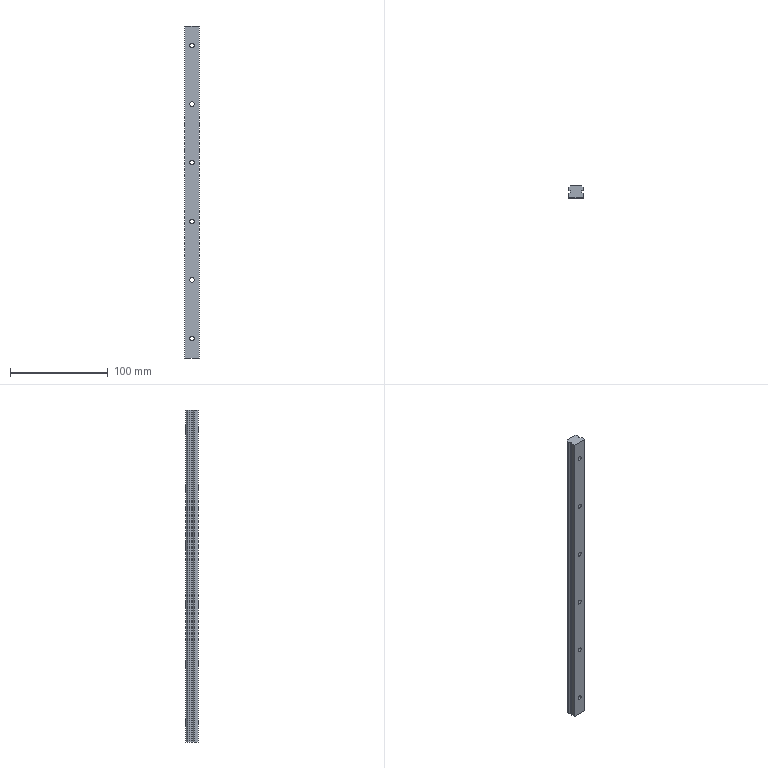Part | NX | features BREP 1 | 1 solid | 46 faces | box 15 x 12.5 x 340 mm | volume 57238 mm3 | cylinder 24 | plane 22 | commonest cylinder face diameters 4.5 x12 7.5 x12
STEP:
#1=CARTESIAN_POINT('',(-78.,48.25,170.));
#2=VERTEX_POINT('',#1);
#3=CARTESIAN_POINT('',(-80.,46.25,170.));
#4=VERTEX_POINT('',#3);
#5=CARTESIAN_POINT('',(-80.,46.25,170.));
#6=DIRECTION('',(-0.7071,-0.7071,0.));
#7=VECTOR('',#6,1000.);
#8=LINE('',#5,#7);
#9=EDGE_CURVE('',#2,#4,#8,.T.);
#10=ORIENTED_EDGE('',*,*,#9,.F.);
#11=CARTESIAN_POINT('',(-78.,48.25,-170.));
#12=VERTEX_POINT('',#11);
#13=CARTESIAN_POINT('',(-78.,48.25,170.));
#14=DIRECTION('',(0.,0.,1.));
#15=VECTOR('',#14,1000.);
#16=LINE('',#13,#15);
#17=EDGE_CURVE('',#12,#2,#16,.T.);
#18=ORIENTED_EDGE('',*,*,#17,.F.);
#19=CARTESIAN_POINT('',(-80.,46.25,-170.));
#20=VERTEX_POINT('',#19);
#21=CARTESIAN_POINT('',(-78.375,47.875,-170.));
#22=DIRECTION('',(0.7071,0.7071,0.));
#23=VECTOR('',#22,1000.);
#24=LINE('',#21,#23);
#25=EDGE_CURVE('',#20,#12,#24,.T.);
#26=ORIENTED_EDGE('',*,*,#25,.F.);
#27=CARTESIAN_POINT('',(-80.,46.25,170.));
#28=DIRECTION('',(0.,0.,-1.));
#29=VECTOR('',#28,1000.);
#30=LINE('',#27,#29);
#31=EDGE_CURVE('',#4,#20,#30,.T.);
#32=ORIENTED_EDGE('',*,*,#31,.F.);
#33=EDGE_LOOP('',(#10,#18,#26,#32));
#34=FACE_BOUND('',#33,.T.);
#35=CARTESIAN_POINT('',(-80.,46.25,170.));
#36=DIRECTION('',(0.7071,-0.7071,0.));
#37=DIRECTION('',(0.,0.,-1.));
#38=AXIS2_PLACEMENT_3D('',#35,#36,#37);
#39=PLANE('',#38);
#40=ADVANCED_FACE('',(#34),#39,.F.);
#41=CARTESIAN_POINT('',(-65.,46.25,170.));
#42=VERTEX_POINT('',#41);
#43=CARTESIAN_POINT('',(-67.,48.25,170.));
#44=VERTEX_POINT('',#43);
#45=CARTESIAN_POINT('',(-67.,48.25,170.));
#46=DIRECTION('',(-0.7071,0.7071,0.));
#47=VECTOR('',#46,1000.);
#48=LINE('',#45,#47);
#49=EDGE_CURVE('',#42,#44,#48,.T.);
#50=ORIENTED_EDGE('',*,*,#49,.F.);
#51=CARTESIAN_POINT('',(-65.,46.25,-170.));
#52=VERTEX_POINT('',#51);
#53=CARTESIAN_POINT('',(-65.,46.25,170.));
#54=DIRECTION('',(0.,0.,1.));
#55=VECTOR('',#54,1000.);
#56=LINE('',#53,#55);
#57=EDGE_CURVE('',#52,#42,#56,.T.);
#58=ORIENTED_EDGE('',*,*,#57,.F.);
#59=CARTESIAN_POINT('',(-67.,48.25,-170.));
#60=VERTEX_POINT('',#59);
#61=CARTESIAN_POINT('',(-66.625,47.875,-170.));
#62=DIRECTION('',(0.7071,-0.7071,0.));
#63=VECTOR('',#62,1000.);
#64=LINE('',#61,#63);
#65=EDGE_CURVE('',#60,#52,#64,.T.);
#66=ORIENTED_EDGE('',*,*,#65,.F.);
#67=CARTESIAN_POINT('',(-67.,48.25,170.));
#68=DIRECTION('',(0.,0.,-1.));
#69=VECTOR('',#68,1000.);
#70=LINE('',#67,#69);
#71=EDGE_CURVE('',#44,#60,#70,.T.);
#72=ORIENTED_EDGE('',*,*,#71,.F.);
#73=EDGE_LOOP('',(#50,#58,#66,#72));
#74=FACE_BOUND('',#73,.T.);
#75=CARTESIAN_POINT('',(-67.,48.25,170.));
#76=DIRECTION('',(-0.7071,-0.7071,0.));
#77=DIRECTION('',(0.,0.,-1.));
#78=AXIS2_PLACEMENT_3D('',#75,#76,#77);
#79=PLANE('',#78);
#80=ADVANCED_FACE('',(#74),#79,.F.);
#81=CARTESIAN_POINT('',(-66.5,42.75,170.));
#82=VERTEX_POINT('',#81);
#83=CARTESIAN_POINT('',(-66.5,41.25,170.));
#84=VERTEX_POINT('',#83);
#85=CARTESIAN_POINT('',(-66.5,41.25,170.));
#86=DIRECTION('',(0.,-1.,0.));
#87=VECTOR('',#86,1000.);
#88=LINE('',#85,#87);
#89=EDGE_CURVE('',#82,#84,#88,.T.);
#90=ORIENTED_EDGE('',*,*,#89,.T.);
#91=CARTESIAN_POINT('',(-66.5,41.25,-170.));
#92=VERTEX_POINT('',#91);
#93=CARTESIAN_POINT('',(-66.5,41.25,-170.));
#94=DIRECTION('',(0.,0.,1.));
#95=VECTOR('',#94,1000.);
#96=LINE('',#93,#95);
#97=EDGE_CURVE('',#92,#84,#96,.T.);
#98=ORIENTED_EDGE('',*,*,#97,.F.);
#99=CARTESIAN_POINT('',(-66.5,42.75,-170.));
#100=VERTEX_POINT('',#99);
#101=CARTESIAN_POINT('',(-66.5,41.25,-170.));
#102=DIRECTION('',(0.,-1.,0.));
#103=VECTOR('',#102,1000.);
#104=LINE('',#101,#103);
#105=EDGE_CURVE('',#100,#92,#104,.T.);
#106=ORIENTED_EDGE('',*,*,#105,.F.);
#107=CARTESIAN_POINT('',(-66.5,42.75,-170.));
#108=DIRECTION('',(0.,0.,1.));
#109=VECTOR('',#108,1000.);
#110=LINE('',#107,#109);
#111=EDGE_CURVE('',#100,#82,#110,.T.);
#112=ORIENTED_EDGE('',*,*,#111,.T.);
#113=EDGE_LOOP('',(#90,#98,#106,#112));
#114=FACE_BOUND('',#113,.T.);
#115=CARTESIAN_POINT('',(-66.5,41.25,-170.));
#116=DIRECTION('',(-1.,0.,0.));
#117=DIRECTION('',(0.,-1.,0.));
#118=AXIS2_PLACEMENT_3D('',#115,#116,#117);
#119=PLANE('',#118);
#120=ADVANCED_FACE('',(#114),#119,.F.);
#121=CARTESIAN_POINT('',(-65.,39.75,170.));
#122=VERTEX_POINT('',#121);
#123=CARTESIAN_POINT('',(-65.,39.75,170.));
#124=DIRECTION('',(0.7071,-0.7071,0.));
#125=VECTOR('',#124,1000.);
#126=LINE('',#123,#125);
#127=EDGE_CURVE('',#84,#122,#126,.T.);
#128=ORIENTED_EDGE('',*,*,#127,.T.);
#129=CARTESIAN_POINT('',(-65.,39.75,-170.));
#130=VERTEX_POINT('',#129);
#131=CARTESIAN_POINT('',(-65.,39.75,-170.));
#132=DIRECTION('',(0.,0.,1.));
#133=VECTOR('',#132,1000.);
#134=LINE('',#131,#133);
#135=EDGE_CURVE('',#130,#122,#134,.T.);
#136=ORIENTED_EDGE('',*,*,#135,.F.);
#137=CARTESIAN_POINT('',(-65.,39.75,-170.));
#138=DIRECTION('',(0.7071,-0.7071,0.));
#139=VECTOR('',#138,1000.);
#140=LINE('',#137,#139);
#141=EDGE_CURVE('',#92,#130,#140,.T.);
#142=ORIENTED_EDGE('',*,*,#141,.F.);
#143=ORIENTED_EDGE('',*,*,#97,.T.);
#144=EDGE_LOOP('',(#128,#136,#142,#143));
#145=FACE_BOUND('',#144,.T.);
#146=CARTESIAN_POINT('',(-65.,39.75,-170.));
#147=DIRECTION('',(-0.7071,-0.7071,0.));
#148=DIRECTION('',(0.7071,-0.7071,0.));
#149=AXIS2_PLACEMENT_3D('',#146,#147,#148);
#150=PLANE('',#149);
#151=ADVANCED_FACE('',(#145),#150,.F.);
#152=CARTESIAN_POINT('',(-65.,44.25,170.));
#153=VERTEX_POINT('',#152);
#154=CARTESIAN_POINT('',(-66.5,42.75,170.));
#155=DIRECTION('',(-0.7071,-0.7071,0.));
#156=VECTOR('',#155,1000.);
#157=LINE('',#154,#156);
#158=EDGE_CURVE('',#153,#82,#157,.T.);
#159=ORIENTED_EDGE('',*,*,#158,.T.);
#160=ORIENTED_EDGE('',*,*,#111,.F.);
#161=CARTESIAN_POINT('',(-65.,44.25,-170.));
#162=VERTEX_POINT('',#161);
#163=CARTESIAN_POINT('',(-66.5,42.75,-170.));
#164=DIRECTION('',(-0.7071,-0.7071,0.));
#165=VECTOR('',#164,1000.);
#166=LINE('',#163,#165);
#167=EDGE_CURVE('',#162,#100,#166,.T.);
#168=ORIENTED_EDGE('',*,*,#167,.F.);
#169=CARTESIAN_POINT('',(-65.,44.25,-170.));
#170=DIRECTION('',(0.,0.,1.));
#171=VECTOR('',#170,1000.);
#172=LINE('',#169,#171);
#173=EDGE_CURVE('',#162,#153,#172,.T.);
#174=ORIENTED_EDGE('',*,*,#173,.T.);
#175=EDGE_LOOP('',(#159,#160,#168,#174));
#176=FACE_BOUND('',#175,.T.);
#177=CARTESIAN_POINT('',(-66.5,42.75,-170.));
#178=DIRECTION('',(-0.7071,0.7071,0.));
#179=DIRECTION('',(-0.7071,-0.7071,0.));
#180=AXIS2_PLACEMENT_3D('',#177,#178,#179);
#181=PLANE('',#180);
#182=ADVANCED_FACE('',(#176),#181,.F.);
#183=CARTESIAN_POINT('',(-80.,39.75,170.));
#184=VERTEX_POINT('',#183);
#185=CARTESIAN_POINT('',(-78.5,41.25,170.));
#186=VERTEX_POINT('',#185);
#187=CARTESIAN_POINT('',(-80.,39.75,170.));
#188=DIRECTION('',(0.7071,0.7071,0.));
#189=VECTOR('',#188,1000.);
#190=LINE('',#187,#189);
#191=EDGE_CURVE('',#184,#186,#190,.T.);
#192=ORIENTED_EDGE('',*,*,#191,.T.);
#193=CARTESIAN_POINT('',(-78.5,41.25,-170.));
#194=VERTEX_POINT('',#193);
#195=CARTESIAN_POINT('',(-78.5,41.25,-170.));
#196=DIRECTION('',(0.,0.,1.));
#197=VECTOR('',#196,1000.);
#198=LINE('',#195,#197);
#199=EDGE_CURVE('',#194,#186,#198,.T.);
#200=ORIENTED_EDGE('',*,*,#199,.F.);
#201=CARTESIAN_POINT('',(-80.,39.75,-170.));
#202=VERTEX_POINT('',#201);
#203=CARTESIAN_POINT('',(-80.,39.75,-170.));
#204=DIRECTION('',(0.7071,0.7071,0.));
#205=VECTOR('',#204,1000.);
#206=LINE('',#203,#205);
#207=EDGE_CURVE('',#202,#194,#206,.T.);
#208=ORIENTED_EDGE('',*,*,#207,.F.);
#209=CARTESIAN_POINT('',(-80.,39.75,-170.));
#210=DIRECTION('',(0.,0.,1.));
#211=VECTOR('',#210,1000.);
#212=LINE('',#209,#211);
#213=EDGE_CURVE('',#202,#184,#212,.T.);
#214=ORIENTED_EDGE('',*,*,#213,.T.);
#215=EDGE_LOOP('',(#192,#200,#208,#214));
#216=FACE_BOUND('',#215,.T.);
#217=CARTESIAN_POINT('',(-80.,39.75,-170.));
#218=DIRECTION('',(0.7071,-0.7071,0.));
#219=DIRECTION('',(0.7071,0.7071,0.));
#220=AXIS2_PLACEMENT_3D('',#217,#218,#219);
#221=PLANE('',#220);
#222=ADVANCED_FACE('',(#216),#221,.F.);
#223=CARTESIAN_POINT('',(-78.5,42.75,170.));
#224=VERTEX_POINT('',#223);
#225=CARTESIAN_POINT('',(-78.5,41.25,170.));
#226=DIRECTION('',(0.,1.,0.));
#227=VECTOR('',#226,1000.);
#228=LINE('',#225,#227);
#229=EDGE_CURVE('',#186,#224,#228,.T.);
#230=ORIENTED_EDGE('',*,*,#229,.T.);
#231=CARTESIAN_POINT('',(-78.5,42.75,-170.));
#232=VERTEX_POINT('',#231);
#233=CARTESIAN_POINT('',(-78.5,42.75,-170.));
#234=DIRECTION('',(0.,0.,1.));
#235=VECTOR('',#234,1000.);
#236=LINE('',#233,#235);
#237=EDGE_CURVE('',#232,#224,#236,.T.);
#238=ORIENTED_EDGE('',*,*,#237,.F.);
#239=CARTESIAN_POINT('',(-78.5,41.25,-170.));
#240=DIRECTION('',(0.,1.,0.));
#241=VECTOR('',#240,1000.);
#242=LINE('',#239,#241);
#243=EDGE_CURVE('',#194,#232,#242,.T.);
#244=ORIENTED_EDGE('',*,*,#243,.F.);
#245=ORIENTED_EDGE('',*,*,#199,.T.);
#246=EDGE_LOOP('',(#230,#238,#244,#245));
#247=FACE_BOUND('',#246,.T.);
#248=CARTESIAN_POINT('',(-78.5,41.25,-170.));
#249=DIRECTION('',(1.,0.,0.));
#250=DIRECTION('',(0.,1.,0.));
#251=AXIS2_PLACEMENT_3D('',#248,#249,#250);
#252=PLANE('',#251);
#253=ADVANCED_FACE('',(#247),#252,.F.);
#254=CARTESIAN_POINT('',(-80.,44.25,170.));
#255=VERTEX_POINT('',#254);
#256=CARTESIAN_POINT('',(-78.5,42.75,170.));
#257=DIRECTION('',(-0.7071,0.7071,0.));
#258=VECTOR('',#257,1000.);
#259=LINE('',#256,#258);
#260=EDGE_CURVE('',#224,#255,#259,.T.);
#261=ORIENTED_EDGE('',*,*,#260,.T.);
#262=CARTESIAN_POINT('',(-80.,44.25,-170.));
#263=VERTEX_POINT('',#262);
#264=CARTESIAN_POINT('',(-80.,44.25,-170.));
#265=DIRECTION('',(0.,0.,1.));
#266=VECTOR('',#265,1000.);
#267=LINE('',#264,#266);
#268=EDGE_CURVE('',#263,#255,#267,.T.);
#269=ORIENTED_EDGE('',*,*,#268,.F.);
#270=CARTESIAN_POINT('',(-78.5,42.75,-170.));
#271=DIRECTION('',(-0.7071,0.7071,0.));
#272=VECTOR('',#271,1000.);
#273=LINE('',#270,#272);
#274=EDGE_CURVE('',#232,#263,#273,.T.);
#275=ORIENTED_EDGE('',*,*,#274,.F.);
#276=ORIENTED_EDGE('',*,*,#237,.T.);
#277=EDGE_LOOP('',(#261,#269,#275,#276));
#278=FACE_BOUND('',#277,.T.);
#279=CARTESIAN_POINT('',(-78.5,42.75,-170.));
#280=DIRECTION('',(0.7071,0.7071,0.));
#281=DIRECTION('',(-0.7071,0.7071,0.));
#282=AXIS2_PLACEMENT_3D('',#279,#280,#281);
#283=PLANE('',#282);
#284=ADVANCED_FACE('',(#278),#283,.F.);
#285=CARTESIAN_POINT('',(-72.5,48.25,86.25));
#286=VERTEX_POINT('',#285);
#287=CARTESIAN_POINT('',(-72.5,42.95,86.25));
#288=VERTEX_POINT('',#287);
#289=CARTESIAN_POINT('',(-72.5,48.25,86.25));
#290=DIRECTION('',(0.,1.,0.));
#291=VECTOR('',#290,1000.);
#292=LINE('',#289,#291);
#293=EDGE_CURVE('',#286,#288,#292,.F.);
#294=ORIENTED_EDGE('',*,*,#293,.T.);
#295=CARTESIAN_POINT('',(-72.5,42.95,93.75));
#296=VERTEX_POINT('',#295);
#297=CARTESIAN_POINT('',(-72.5,42.95,90.));
#298=DIRECTION('',(0.,1.,0.));
#299=DIRECTION('',(0.,0.,1.));
#300=AXIS2_PLACEMENT_3D('',#297,#298,#299);
#301=CIRCLE('',#300,3.75);
#302=EDGE_CURVE('',#296,#288,#301,.T.);
#303=ORIENTED_EDGE('',*,*,#302,.F.);
#304=CARTESIAN_POINT('',(-72.5,48.25,93.75));
#305=VERTEX_POINT('',#304);
#306=CARTESIAN_POINT('',(-72.5,48.25,93.75));
#307=DIRECTION('',(0.,1.,0.));
#308=VECTOR('',#307,1000.);
#309=LINE('',#306,#308);
#310=EDGE_CURVE('',#305,#296,#309,.F.);
#311=ORIENTED_EDGE('',*,*,#310,.F.);
#312=CARTESIAN_POINT('',(-72.5,48.25,90.));
#313=DIRECTION('',(0.,1.,0.));
#314=DIRECTION('',(0.,0.,1.));
#315=AXIS2_PLACEMENT_3D('',#312,#313,#314);
#316=CIRCLE('',#315,3.75);
#317=EDGE_CURVE('',#305,#286,#316,.T.);
#318=ORIENTED_EDGE('',*,*,#317,.T.);
#319=EDGE_LOOP('',(#294,#303,#311,#318));
#320=FACE_BOUND('',#319,.T.);
#321=CARTESIAN_POINT('',(-72.5,48.25,90.));
#322=DIRECTION('',(0.,1.,0.));
#323=DIRECTION('',(0.,0.,1.));
#324=AXIS2_PLACEMENT_3D('',#321,#322,#323);
#325=CYLINDRICAL_SURFACE('',#324,3.75);
#326=ADVANCED_FACE('',(#320),#325,.F.);
#327=ORIENTED_EDGE('',*,*,#302,.T.);
#328=CARTESIAN_POINT('',(-72.5,42.95,90.));
#329=DIRECTION('',(0.,1.,0.));
#330=DIRECTION('',(0.,0.,1.));
#331=AXIS2_PLACEMENT_3D('',#328,#329,#330);
#332=CIRCLE('',#331,3.75);
#333=EDGE_CURVE('',#288,#296,#332,.T.);
#334=ORIENTED_EDGE('',*,*,#333,.T.);
#335=EDGE_LOOP('',(#327,#334));
#336=FACE_BOUND('',#335,.T.);
#337=CARTESIAN_POINT('',(-72.5,42.95,92.25));
#338=VERTEX_POINT('',#337);
#339=CARTESIAN_POINT('',(-72.5,42.95,87.75));
#340=VERTEX_POINT('',#339);
#341=CARTESIAN_POINT('',(-72.5,42.95,90.));
#342=DIRECTION('',(0.,1.,0.));
#343=DIRECTION('',(0.,0.,1.));
#344=AXIS2_PLACEMENT_3D('',#341,#342,#343);
#345=CIRCLE('',#344,2.25);
#346=EDGE_CURVE('',#338,#340,#345,.T.);
#347=ORIENTED_EDGE('',*,*,#346,.F.);
#348=CARTESIAN_POINT('',(-72.5,42.95,90.));
#349=DIRECTION('',(0.,1.,0.));
#350=DIRECTION('',(0.,0.,1.));
#351=AXIS2_PLACEMENT_3D('',#348,#349,#350);
#352=CIRCLE('',#351,2.25);
#353=EDGE_CURVE('',#340,#338,#352,.T.);
#354=ORIENTED_EDGE('',*,*,#353,.F.);
#355=EDGE_LOOP('',(#347,#354));
#356=FACE_BOUND('',#355,.T.);
#357=CARTESIAN_POINT('',(-70.25,42.95,90.));
#358=DIRECTION('',(0.,-1.,0.));
#359=DIRECTION('',(0.,0.,-1.));
#360=AXIS2_PLACEMENT_3D('',#357,#358,#359);
#361=PLANE('',#360);
#362=ADVANCED_FACE('',(#336,#356),#361,.F.);
#363=CARTESIAN_POINT('',(-72.5,35.75,87.75));
#364=VERTEX_POINT('',#363);
#365=CARTESIAN_POINT('',(-72.5,48.25,87.75));
#366=DIRECTION('',(0.,1.,0.));
#367=VECTOR('',#366,1000.);
#368=LINE('',#365,#367);
#369=EDGE_CURVE('',#340,#364,#368,.F.);
#370=ORIENTED_EDGE('',*,*,#369,.T.);
#371=CARTESIAN_POINT('',(-72.5,35.75,92.25));
#372=VERTEX_POINT('',#371);
#373=CARTESIAN_POINT('',(-72.5,35.75,90.));
#374=DIRECTION('',(0.,1.,0.));
#375=DIRECTION('',(0.,0.,1.));
#376=AXIS2_PLACEMENT_3D('',#373,#374,#375);
#377=CIRCLE('',#376,2.25);
#378=EDGE_CURVE('',#372,#364,#377,.T.);
#379=ORIENTED_EDGE('',*,*,#378,.F.);
#380=CARTESIAN_POINT('',(-72.5,48.25,92.25));
#381=DIRECTION('',(0.,1.,0.));
#382=VECTOR('',#381,1000.);
#383=LINE('',#380,#382);
#384=EDGE_CURVE('',#338,#372,#383,.F.);
#385=ORIENTED_EDGE('',*,*,#384,.F.);
#386=ORIENTED_EDGE('',*,*,#346,.T.);
#387=EDGE_LOOP('',(#370,#379,#385,#386));
#388=FACE_BOUND('',#387,.T.);
#389=CARTESIAN_POINT('',(-72.5,48.25,90.));
#390=DIRECTION('',(0.,1.,0.));
#391=DIRECTION('',(0.,0.,1.));
#392=AXIS2_PLACEMENT_3D('',#389,#390,#391);
#393=CYLINDRICAL_SURFACE('',#392,2.25);
#394=ADVANCED_FACE('',(#388),#393,.F.);
#395=CARTESIAN_POINT('',(-72.5,48.25,146.25));
#396=VERTEX_POINT('',#395);
#397=CARTESIAN_POINT('',(-72.5,42.95,146.25));
#398=VERTEX_POINT('',#397);
#399=CARTESIAN_POINT('',(-72.5,48.25,146.25));
#400=DIRECTION('',(0.,1.,0.));
#401=VECTOR('',#400,1000.);
#402=LINE('',#399,#401);
#403=EDGE_CURVE('',#396,#398,#402,.F.);
#404=ORIENTED_EDGE('',*,*,#403,.T.);
#405=CARTESIAN_POINT('',(-72.5,42.95,153.75));
#406=VERTEX_POINT('',#405);
#407=CARTESIAN_POINT('',(-72.5,42.95,150.));
#408=DIRECTION('',(0.,1.,0.));
#409=DIRECTION('',(0.,0.,1.));
#410=AXIS2_PLACEMENT_3D('',#407,#408,#409);
#411=CIRCLE('',#410,3.75);
#412=EDGE_CURVE('',#406,#398,#411,.T.);
#413=ORIENTED_EDGE('',*,*,#412,.F.);
#414=CARTESIAN_POINT('',(-72.5,48.25,153.75));
#415=VERTEX_POINT('',#414);
#416=CARTESIAN_POINT('',(-72.5,48.25,153.75));
#417=DIRECTION('',(0.,1.,0.));
#418=VECTOR('',#417,1000.);
#419=LINE('',#416,#418);
#420=EDGE_CURVE('',#415,#406,#419,.F.);
#421=ORIENTED_EDGE('',*,*,#420,.F.);
#422=CARTESIAN_POINT('',(-72.5,48.25,150.));
#423=DIRECTION('',(0.,1.,0.));
#424=DIRECTION('',(0.,0.,1.));
#425=AXIS2_PLACEMENT_3D('',#422,#423,#424);
#426=CIRCLE('',#425,3.75);
#427=EDGE_CURVE('',#415,#396,#426,.T.);
#428=ORIENTED_EDGE('',*,*,#427,.T.);
#429=EDGE_LOOP('',(#404,#413,#421,#428));
#430=FACE_BOUND('',#429,.T.);
#431=CARTESIAN_POINT('',(-72.5,48.25,150.));
#432=DIRECTION('',(0.,1.,0.));
#433=DIRECTION('',(0.,0.,1.));
#434=AXIS2_PLACEMENT_3D('',#431,#432,#433);
#435=CYLINDRICAL_SURFACE('',#434,3.75);
#436=ADVANCED_FACE('',(#430),#435,.F.);
#437=ORIENTED_EDGE('',*,*,#412,.T.);
#438=CARTESIAN_POINT('',(-72.5,42.95,150.));
#439=DIRECTION('',(0.,1.,0.));
#440=DIRECTION('',(0.,0.,1.));
#441=AXIS2_PLACEMENT_3D('',#438,#439,#440);
#442=CIRCLE('',#441,3.75);
#443=EDGE_CURVE('',#398,#406,#442,.T.);
#444=ORIENTED_EDGE('',*,*,#443,.T.);
#445=EDGE_LOOP('',(#437,#444));
#446=FACE_BOUND('',#445,.T.);
#447=CARTESIAN_POINT('',(-72.5,42.95,152.25));
#448=VERTEX_POINT('',#447);
#449=CARTESIAN_POINT('',(-72.5,42.95,147.75));
#450=VERTEX_POINT('',#449);
#451=CARTESIAN_POINT('',(-72.5,42.95,150.));
#452=DIRECTION('',(0.,1.,0.));
#453=DIRECTION('',(0.,0.,1.));
#454=AXIS2_PLACEMENT_3D('',#451,#452,#453);
#455=CIRCLE('',#454,2.25);
#456=EDGE_CURVE('',#448,#450,#455,.T.);
#457=ORIENTED_EDGE('',*,*,#456,.F.);
#458=CARTESIAN_POINT('',(-72.5,42.95,150.));
#459=DIRECTION('',(0.,1.,0.));
#460=DIRECTION('',(0.,0.,1.));
#461=AXIS2_PLACEMENT_3D('',#458,#459,#460);
#462=CIRCLE('',#461,2.25);
#463=EDGE_CURVE('',#450,#448,#462,.T.);
#464=ORIENTED_EDGE('',*,*,#463,.F.);
#465=EDGE_LOOP('',(#457,#464));
#466=FACE_BOUND('',#465,.T.);
#467=CARTESIAN_POINT('',(-70.25,42.95,150.));
#468=DIRECTION('',(0.,-1.,0.));
#469=DIRECTION('',(0.,0.,-1.));
#470=AXIS2_PLACEMENT_3D('',#467,#468,#469);
#471=PLANE('',#470);
#472=ADVANCED_FACE('',(#446,#466),#471,.F.);
#473=CARTESIAN_POINT('',(-72.5,35.75,147.75));
#474=VERTEX_POINT('',#473);
#475=CARTESIAN_POINT('',(-72.5,48.25,147.75));
#476=DIRECTION('',(0.,1.,0.));
#477=VECTOR('',#476,1000.);
#478=LINE('',#475,#477);
#479=EDGE_CURVE('',#450,#474,#478,.F.);
#480=ORIENTED_EDGE('',*,*,#479,.T.);
#481=CARTESIAN_POINT('',(-72.5,35.75,152.25));
#482=VERTEX_POINT('',#481);
#483=CARTESIAN_POINT('',(-72.5,35.75,150.));
#484=DIRECTION('',(0.,1.,0.));
#485=DIRECTION('',(0.,0.,1.));
#486=AXIS2_PLACEMENT_3D('',#483,#484,#485);
#487=CIRCLE('',#486,2.25);
#488=EDGE_CURVE('',#482,#474,#487,.T.);
#489=ORIENTED_EDGE('',*,*,#488,.F.);
#490=CARTESIAN_POINT('',(-72.5,48.25,152.25));
#491=DIRECTION('',(0.,1.,0.));
#492=VECTOR('',#491,1000.);
#493=LINE('',#490,#492);
#494=EDGE_CURVE('',#448,#482,#493,.F.);
#495=ORIENTED_EDGE('',*,*,#494,.F.);
#496=ORIENTED_EDGE('',*,*,#456,.T.);
#497=EDGE_LOOP('',(#480,#489,#495,#496));
#498=FACE_BOUND('',#497,.T.);
#499=CARTESIAN_POINT('',(-72.5,48.25,150.));
#500=DIRECTION('',(0.,1.,0.));
#501=DIRECTION('',(0.,0.,1.));
#502=AXIS2_PLACEMENT_3D('',#499,#500,#501);
#503=CYLINDRICAL_SURFACE('',#502,2.25);
#504=ADVANCED_FACE('',(#498),#503,.F.);
#505=CARTESIAN_POINT('',(-80.,48.25,-170.));
#506=DIRECTION('',(-1.,0.,0.));
#507=VECTOR('',#506,1000.);
#508=LINE('',#505,#507);
#509=EDGE_CURVE('',#60,#12,#508,.T.);
#510=ORIENTED_EDGE('',*,*,#509,.F.);
#511=ORIENTED_EDGE('',*,*,#65,.T.);
#512=CARTESIAN_POINT('',(-65.,35.75,-170.));
#513=DIRECTION('',(0.,1.,0.));
#514=VECTOR('',#513,1000.);
#515=LINE('',#512,#514);
#516=EDGE_CURVE('',#162,#52,#515,.T.);
#517=ORIENTED_EDGE('',*,*,#516,.F.);
#518=ORIENTED_EDGE('',*,*,#167,.T.);
#519=ORIENTED_EDGE('',*,*,#105,.T.);
#520=ORIENTED_EDGE('',*,*,#141,.T.);
#521=CARTESIAN_POINT('',(-65.,35.75,-170.));
#522=VERTEX_POINT('',#521);
#523=CARTESIAN_POINT('',(-65.,35.75,-170.));
#524=DIRECTION('',(0.,1.,0.));
#525=VECTOR('',#524,1000.);
#526=LINE('',#523,#525);
#527=EDGE_CURVE('',#522,#130,#526,.T.);
#528=ORIENTED_EDGE('',*,*,#527,.F.);
#529=CARTESIAN_POINT('',(-80.,35.75,-170.));
#530=VERTEX_POINT('',#529);
#531=CARTESIAN_POINT('',(-80.,35.75,-170.));
#532=DIRECTION('',(1.,0.,0.));
#533=VECTOR('',#532,1000.);
#534=LINE('',#531,#533);
#535=EDGE_CURVE('',#530,#522,#534,.T.);
#536=ORIENTED_EDGE('',*,*,#535,.F.);
#537=CARTESIAN_POINT('',(-80.,35.75,-170.));
#538=DIRECTION('',(0.,-1.,0.));
#539=VECTOR('',#538,1000.);
#540=LINE('',#537,#539);
#541=EDGE_CURVE('',#202,#530,#540,.T.);
#542=ORIENTED_EDGE('',*,*,#541,.F.);
#543=ORIENTED_EDGE('',*,*,#207,.T.);
#544=ORIENTED_EDGE('',*,*,#243,.T.);
#545=ORIENTED_EDGE('',*,*,#274,.T.);
#546=CARTESIAN_POINT('',(-80.,35.75,-170.));
#547=DIRECTION('',(0.,-1.,0.));
#548=VECTOR('',#547,1000.);
#549=LINE('',#546,#548);
#550=EDGE_CURVE('',#20,#263,#549,.T.);
#551=ORIENTED_EDGE('',*,*,#550,.F.);
#552=ORIENTED_EDGE('',*,*,#25,.T.);
#553=EDGE_LOOP('',(#510,#511,#517,#518,#519,#520,#528,#536,#542,#543,#544,#545,#551,#552));
#554=FACE_BOUND('',#553,.T.);
#555=CARTESIAN_POINT('',(-72.5,42.,-170.));
#556=DIRECTION('',(0.,0.,-1.));
#557=DIRECTION('',(-1.,0.,0.));
#558=AXIS2_PLACEMENT_3D('',#555,#556,#557);
#559=PLANE('',#558);
#560=ADVANCED_FACE('',(#554),#559,.T.);
#561=CARTESIAN_POINT('',(-65.,35.75,170.));
#562=DIRECTION('',(0.,1.,0.));
#563=VECTOR('',#562,1000.);
#564=LINE('',#561,#563);
#565=EDGE_CURVE('',#153,#42,#564,.T.);
#566=ORIENTED_EDGE('',*,*,#565,.T.);
#567=ORIENTED_EDGE('',*,*,#49,.T.);
#568=CARTESIAN_POINT('',(-80.,48.25,170.));
#569=DIRECTION('',(-1.,0.,0.));
#570=VECTOR('',#569,1000.);
#571=LINE('',#568,#570);
#572=EDGE_CURVE('',#44,#2,#571,.T.);
#573=ORIENTED_EDGE('',*,*,#572,.T.);
#574=ORIENTED_EDGE('',*,*,#9,.T.);
#575=CARTESIAN_POINT('',(-80.,35.75,170.));
#576=DIRECTION('',(0.,-1.,0.));
#577=VECTOR('',#576,1000.);
#578=LINE('',#575,#577);
#579=EDGE_CURVE('',#4,#255,#578,.T.);
#580=ORIENTED_EDGE('',*,*,#579,.T.);
#581=ORIENTED_EDGE('',*,*,#260,.F.);
#582=ORIENTED_EDGE('',*,*,#229,.F.);
#583=ORIENTED_EDGE('',*,*,#191,.F.);
#584=CARTESIAN_POINT('',(-80.,35.75,170.));
#585=VERTEX_POINT('',#584);
#586=CARTESIAN_POINT('',(-80.,35.75,170.));
#587=DIRECTION('',(0.,-1.,0.));
#588=VECTOR('',#587,1000.);
#589=LINE('',#586,#588);
#590=EDGE_CURVE('',#184,#585,#589,.T.);
#591=ORIENTED_EDGE('',*,*,#590,.T.);
#592=CARTESIAN_POINT('',(-65.,35.75,170.));
#593=VERTEX_POINT('',#592);
#594=CARTESIAN_POINT('',(-80.,35.75,170.));
#595=DIRECTION('',(1.,0.,0.));
#596=VECTOR('',#595,1000.);
#597=LINE('',#594,#596);
#598=EDGE_CURVE('',#585,#593,#597,.T.);
#599=ORIENTED_EDGE('',*,*,#598,.T.);
#600=CARTESIAN_POINT('',(-65.,35.75,170.));
#601=DIRECTION('',(0.,1.,0.));
#602=VECTOR('',#601,1000.);
#603=LINE('',#600,#602);
#604=EDGE_CURVE('',#593,#122,#603,.T.);
#605=ORIENTED_EDGE('',*,*,#604,.T.);
#606=ORIENTED_EDGE('',*,*,#127,.F.);
#607=ORIENTED_EDGE('',*,*,#89,.F.);
#608=ORIENTED_EDGE('',*,*,#158,.F.);
#609=EDGE_LOOP('',(#566,#567,#573,#574,#580,#581,#582,#583,#591,#599,#605,#606,#607,#608));
#610=FACE_BOUND('',#609,.T.);
#611=CARTESIAN_POINT('',(-72.5,42.,170.));
#612=DIRECTION('',(0.,0.,-1.));
#613=DIRECTION('',(-1.,0.,0.));
#614=AXIS2_PLACEMENT_3D('',#611,#612,#613);
#615=PLANE('',#614);
#616=ADVANCED_FACE('',(#610),#615,.F.);
#617=CARTESIAN_POINT('',(-72.5,35.75,-147.75));
#618=VERTEX_POINT('',#617);
#619=CARTESIAN_POINT('',(-72.5,35.75,-152.25));
#620=VERTEX_POINT('',#619);
#621=CARTESIAN_POINT('',(-72.5,35.75,-150.));
#622=DIRECTION('',(0.,1.,0.));
#623=DIRECTION('',(0.,0.,1.));
#624=AXIS2_PLACEMENT_3D('',#621,#622,#623);
#625=CIRCLE('',#624,2.25);
#626=EDGE_CURVE('',#618,#620,#625,.T.);
#627=ORIENTED_EDGE('',*,*,#626,.T.);
#628=CARTESIAN_POINT('',(-72.5,35.75,-150.));
#629=DIRECTION('',(0.,1.,0.));
#630=DIRECTION('',(0.,0.,1.));
#631=AXIS2_PLACEMENT_3D('',#628,#629,#630);
#632=CIRCLE('',#631,2.25);
#633=EDGE_CURVE('',#620,#618,#632,.T.);
#634=ORIENTED_EDGE('',*,*,#633,.T.);
#635=EDGE_LOOP('',(#627,#634));
#636=FACE_BOUND('',#635,.T.);
#637=CARTESIAN_POINT('',(-72.5,35.75,-87.75));
#638=VERTEX_POINT('',#637);
#639=CARTESIAN_POINT('',(-72.5,35.75,-92.25));
#640=VERTEX_POINT('',#639);
#641=CARTESIAN_POINT('',(-72.5,35.75,-90.));
#642=DIRECTION('',(0.,1.,0.));
#643=DIRECTION('',(0.,0.,1.));
#644=AXIS2_PLACEMENT_3D('',#641,#642,#643);
#645=CIRCLE('',#644,2.25);
#646=EDGE_CURVE('',#638,#640,#645,.T.);
#647=ORIENTED_EDGE('',*,*,#646,.T.);
#648=CARTESIAN_POINT('',(-72.5,35.75,-90.));
#649=DIRECTION('',(0.,1.,0.));
#650=DIRECTION('',(0.,0.,1.));
#651=AXIS2_PLACEMENT_3D('',#648,#649,#650);
#652=CIRCLE('',#651,2.25);
#653=EDGE_CURVE('',#640,#638,#652,.T.);
#654=ORIENTED_EDGE('',*,*,#653,.T.);
#655=EDGE_LOOP('',(#647,#654));
#656=FACE_BOUND('',#655,.T.);
#657=CARTESIAN_POINT('',(-72.5,35.75,-27.75));
#658=VERTEX_POINT('',#657);
#659=CARTESIAN_POINT('',(-72.5,35.75,-32.25));
#660=VERTEX_POINT('',#659);
#661=CARTESIAN_POINT('',(-72.5,35.75,-30.));
#662=DIRECTION('',(0.,1.,0.));
#663=DIRECTION('',(0.,0.,1.));
#664=AXIS2_PLACEMENT_3D('',#661,#662,#663);
#665=CIRCLE('',#664,2.25);
#666=EDGE_CURVE('',#658,#660,#665,.T.);
#667=ORIENTED_EDGE('',*,*,#666,.T.);
#668=CARTESIAN_POINT('',(-72.5,35.75,-30.));
#669=DIRECTION('',(0.,1.,0.));
#670=DIRECTION('',(0.,0.,1.));
#671=AXIS2_PLACEMENT_3D('',#668,#669,#670);
#672=CIRCLE('',#671,2.25);
#673=EDGE_CURVE('',#660,#658,#672,.T.);
#674=ORIENTED_EDGE('',*,*,#673,.T.);
#675=EDGE_LOOP('',(#667,#674));
#676=FACE_BOUND('',#675,.T.);
#677=CARTESIAN_POINT('',(-72.5,35.75,32.25));
#678=VERTEX_POINT('',#677);
#679=CARTESIAN_POINT('',(-72.5,35.75,27.75));
#680=VERTEX_POINT('',#679);
#681=CARTESIAN_POINT('',(-72.5,35.75,30.));
#682=DIRECTION('',(0.,1.,0.));
#683=DIRECTION('',(0.,0.,1.));
#684=AXIS2_PLACEMENT_3D('',#681,#682,#683);
#685=CIRCLE('',#684,2.25);
#686=EDGE_CURVE('',#678,#680,#685,.T.);
#687=ORIENTED_EDGE('',*,*,#686,.T.);
#688=CARTESIAN_POINT('',(-72.5,35.75,30.));
#689=DIRECTION('',(0.,1.,0.));
#690=DIRECTION('',(0.,0.,1.));
#691=AXIS2_PLACEMENT_3D('',#688,#689,#690);
#692=CIRCLE('',#691,2.25);
#693=EDGE_CURVE('',#680,#678,#692,.T.);
#694=ORIENTED_EDGE('',*,*,#693,.T.);
#695=EDGE_LOOP('',(#687,#694));
#696=FACE_BOUND('',#695,.T.);
#697=ORIENTED_EDGE('',*,*,#535,.T.);
#698=CARTESIAN_POINT('',(-65.,35.75,170.));
#699=DIRECTION('',(0.,0.,-1.));
#700=VECTOR('',#699,1000.);
#701=LINE('',#698,#700);
#702=EDGE_CURVE('',#593,#522,#701,.T.);
#703=ORIENTED_EDGE('',*,*,#702,.F.);
#704=ORIENTED_EDGE('',*,*,#598,.F.);
#705=CARTESIAN_POINT('',(-80.,35.75,170.));
#706=DIRECTION('',(0.,0.,-1.));
#707=VECTOR('',#706,1000.);
#708=LINE('',#705,#707);
#709=EDGE_CURVE('',#585,#530,#708,.T.);
#710=ORIENTED_EDGE('',*,*,#709,.T.);
#711=EDGE_LOOP('',(#697,#703,#704,#710));
#712=FACE_BOUND('',#711,.T.);
#713=ORIENTED_EDGE('',*,*,#488,.T.);
#714=CARTESIAN_POINT('',(-72.5,35.75,150.));
#715=DIRECTION('',(0.,1.,0.));
#716=DIRECTION('',(0.,0.,1.));
#717=AXIS2_PLACEMENT_3D('',#714,#715,#716);
#718=CIRCLE('',#717,2.25);
#719=EDGE_CURVE('',#474,#482,#718,.T.);
#720=ORIENTED_EDGE('',*,*,#719,.T.);
#721=EDGE_LOOP('',(#713,#720));
#722=FACE_BOUND('',#721,.T.);
#723=ORIENTED_EDGE('',*,*,#378,.T.);
#724=CARTESIAN_POINT('',(-72.5,35.75,90.));
#725=DIRECTION('',(0.,1.,0.));
#726=DIRECTION('',(0.,0.,1.));
#727=AXIS2_PLACEMENT_3D('',#724,#725,#726);
#728=CIRCLE('',#727,2.25);
#729=EDGE_CURVE('',#364,#372,#728,.T.);
#730=ORIENTED_EDGE('',*,*,#729,.T.);
#731=EDGE_LOOP('',(#723,#730));
#732=FACE_BOUND('',#731,.T.);
#733=CARTESIAN_POINT('',(-80.,35.75,170.));
#734=DIRECTION('',(0.,1.,0.));
#735=DIRECTION('',(0.,0.,1.));
#736=AXIS2_PLACEMENT_3D('',#733,#734,#735);
#737=PLANE('',#736);
#738=ADVANCED_FACE('',(#636,#656,#676,#696,#712,#722,#732),#737,.F.);
#739=ORIENTED_EDGE('',*,*,#590,.F.);
#740=ORIENTED_EDGE('',*,*,#213,.F.);
#741=ORIENTED_EDGE('',*,*,#541,.T.);
#742=ORIENTED_EDGE('',*,*,#709,.F.);
#743=EDGE_LOOP('',(#739,#740,#741,#742));
#744=FACE_BOUND('',#743,.T.);
#745=CARTESIAN_POINT('',(-80.,35.75,170.));
#746=DIRECTION('',(1.,0.,0.));
#747=DIRECTION('',(0.,0.,-1.));
#748=AXIS2_PLACEMENT_3D('',#745,#746,#747);
#749=PLANE('',#748);
#750=ADVANCED_FACE('',(#744),#749,.F.);
#751=CARTESIAN_POINT('',(-72.5,48.25,-146.25));
#752=VERTEX_POINT('',#751);
#753=CARTESIAN_POINT('',(-72.5,48.25,-153.75));
#754=VERTEX_POINT('',#753);
#755=CARTESIAN_POINT('',(-72.5,48.25,-150.));
#756=DIRECTION('',(0.,1.,0.));
#757=DIRECTION('',(0.,0.,1.));
#758=AXIS2_PLACEMENT_3D('',#755,#756,#757);
#759=CIRCLE('',#758,3.75);
#760=EDGE_CURVE('',#752,#754,#759,.T.);
#761=ORIENTED_EDGE('',*,*,#760,.F.);
#762=CARTESIAN_POINT('',(-72.5,48.25,-150.));
#763=DIRECTION('',(0.,1.,0.));
#764=DIRECTION('',(0.,0.,1.));
#765=AXIS2_PLACEMENT_3D('',#762,#763,#764);
#766=CIRCLE('',#765,3.75);
#767=EDGE_CURVE('',#754,#752,#766,.T.);
#768=ORIENTED_EDGE('',*,*,#767,.F.);
#769=EDGE_LOOP('',(#761,#768));
#770=FACE_BOUND('',#769,.T.);
#771=CARTESIAN_POINT('',(-72.5,48.25,-86.25));
#772=VERTEX_POINT('',#771);
#773=CARTESIAN_POINT('',(-72.5,48.25,-93.75));
#774=VERTEX_POINT('',#773);
#775=CARTESIAN_POINT('',(-72.5,48.25,-90.));
#776=DIRECTION('',(0.,1.,0.));
#777=DIRECTION('',(0.,0.,1.));
#778=AXIS2_PLACEMENT_3D('',#775,#776,#777);
#779=CIRCLE('',#778,3.75);
#780=EDGE_CURVE('',#772,#774,#779,.T.);
#781=ORIENTED_EDGE('',*,*,#780,.F.);
#782=CARTESIAN_POINT('',(-72.5,48.25,-90.));
#783=DIRECTION('',(0.,1.,0.));
#784=DIRECTION('',(0.,0.,1.));
#785=AXIS2_PLACEMENT_3D('',#782,#783,#784);
#786=CIRCLE('',#785,3.75);
#787=EDGE_CURVE('',#774,#772,#786,.T.);
#788=ORIENTED_EDGE('',*,*,#787,.F.);
#789=EDGE_LOOP('',(#781,#788));
#790=FACE_BOUND('',#789,.T.);
#791=CARTESIAN_POINT('',(-72.5,48.25,-26.25));
#792=VERTEX_POINT('',#791);
#793=CARTESIAN_POINT('',(-72.5,48.25,-33.75));
#794=VERTEX_POINT('',#793);
#795=CARTESIAN_POINT('',(-72.5,48.25,-30.));
#796=DIRECTION('',(0.,1.,0.));
#797=DIRECTION('',(0.,0.,1.));
#798=AXIS2_PLACEMENT_3D('',#795,#796,#797);
#799=CIRCLE('',#798,3.75);
#800=EDGE_CURVE('',#792,#794,#799,.T.);
#801=ORIENTED_EDGE('',*,*,#800,.F.);
#802=CARTESIAN_POINT('',(-72.5,48.25,-30.));
#803=DIRECTION('',(0.,1.,0.));
#804=DIRECTION('',(0.,0.,1.));
#805=AXIS2_PLACEMENT_3D('',#802,#803,#804);
#806=CIRCLE('',#805,3.75);
#807=EDGE_CURVE('',#794,#792,#806,.T.);
#808=ORIENTED_EDGE('',*,*,#807,.F.);
#809=EDGE_LOOP('',(#801,#808));
#810=FACE_BOUND('',#809,.T.);
#811=CARTESIAN_POINT('',(-72.5,48.25,33.75));
#812=VERTEX_POINT('',#811);
#813=CARTESIAN_POINT('',(-72.5,48.25,26.25));
#814=VERTEX_POINT('',#813);
#815=CARTESIAN_POINT('',(-72.5,48.25,30.));
#816=DIRECTION('',(0.,1.,0.));
#817=DIRECTION('',(0.,0.,1.));
#818=AXIS2_PLACEMENT_3D('',#815,#816,#817);
#819=CIRCLE('',#818,3.75);
#820=EDGE_CURVE('',#812,#814,#819,.T.);
#821=ORIENTED_EDGE('',*,*,#820,.F.);
#822=CARTESIAN_POINT('',(-72.5,48.25,30.));
#823=DIRECTION('',(0.,1.,0.));
#824=DIRECTION('',(0.,0.,1.));
#825=AXIS2_PLACEMENT_3D('',#822,#823,#824);
#826=CIRCLE('',#825,3.75);
#827=EDGE_CURVE('',#814,#812,#826,.T.);
#828=ORIENTED_EDGE('',*,*,#827,.F.);
#829=EDGE_LOOP('',(#821,#828));
#830=FACE_BOUND('',#829,.T.);
#831=ORIENTED_EDGE('',*,*,#572,.F.);
#832=ORIENTED_EDGE('',*,*,#71,.T.);
#833=ORIENTED_EDGE('',*,*,#509,.T.);
#834=ORIENTED_EDGE('',*,*,#17,.T.);
#835=EDGE_LOOP('',(#831,#832,#833,#834));
#836=FACE_BOUND('',#835,.T.);
#837=ORIENTED_EDGE('',*,*,#427,.F.);
#838=CARTESIAN_POINT('',(-72.5,48.25,150.));
#839=DIRECTION('',(0.,1.,0.));
#840=DIRECTION('',(0.,0.,1.));
#841=AXIS2_PLACEMENT_3D('',#838,#839,#840);
#842=CIRCLE('',#841,3.75);
#843=EDGE_CURVE('',#396,#415,#842,.T.);
#844=ORIENTED_EDGE('',*,*,#843,.F.);
#845=EDGE_LOOP('',(#837,#844));
#846=FACE_BOUND('',#845,.T.);
#847=ORIENTED_EDGE('',*,*,#317,.F.);
#848=CARTESIAN_POINT('',(-72.5,48.25,90.));
#849=DIRECTION('',(0.,1.,0.));
#850=DIRECTION('',(0.,0.,1.));
#851=AXIS2_PLACEMENT_3D('',#848,#849,#850);
#852=CIRCLE('',#851,3.75);
#853=EDGE_CURVE('',#286,#305,#852,.T.);
#854=ORIENTED_EDGE('',*,*,#853,.F.);
#855=EDGE_LOOP('',(#847,#854));
#856=FACE_BOUND('',#855,.T.);
#857=CARTESIAN_POINT('',(-80.,48.25,170.));
#858=DIRECTION('',(0.,-1.,0.));
#859=DIRECTION('',(0.,0.,-1.));
#860=AXIS2_PLACEMENT_3D('',#857,#858,#859);
#861=PLANE('',#860);
#862=ADVANCED_FACE('',(#770,#790,#810,#830,#836,#846,#856),#861,.F.);
#863=ORIENTED_EDGE('',*,*,#527,.T.);
#864=ORIENTED_EDGE('',*,*,#135,.T.);
#865=ORIENTED_EDGE('',*,*,#604,.F.);
#866=ORIENTED_EDGE('',*,*,#702,.T.);
#867=EDGE_LOOP('',(#863,#864,#865,#866));
#868=FACE_BOUND('',#867,.T.);
#869=CARTESIAN_POINT('',(-65.,35.75,170.));
#870=DIRECTION('',(-1.,0.,0.));
#871=DIRECTION('',(0.,0.,1.));
#872=AXIS2_PLACEMENT_3D('',#869,#870,#871);
#873=PLANE('',#872);
#874=ADVANCED_FACE('',(#868),#873,.F.);
#875=CARTESIAN_POINT('',(-72.5,42.95,27.75));
#876=VERTEX_POINT('',#875);
#877=CARTESIAN_POINT('',(-72.5,48.25,27.75));
#878=DIRECTION('',(0.,1.,0.));
#879=VECTOR('',#878,1000.);
#880=LINE('',#877,#879);
#881=EDGE_CURVE('',#876,#680,#880,.F.);
#882=ORIENTED_EDGE('',*,*,#881,.T.);
#883=ORIENTED_EDGE('',*,*,#686,.F.);
#884=CARTESIAN_POINT('',(-72.5,42.95,32.25));
#885=VERTEX_POINT('',#884);
#886=CARTESIAN_POINT('',(-72.5,48.25,32.25));
#887=DIRECTION('',(0.,1.,0.));
#888=VECTOR('',#887,1000.);
#889=LINE('',#886,#888);
#890=EDGE_CURVE('',#885,#678,#889,.F.);
#891=ORIENTED_EDGE('',*,*,#890,.F.);
#892=CARTESIAN_POINT('',(-72.5,42.95,30.));
#893=DIRECTION('',(0.,1.,0.));
#894=DIRECTION('',(0.,0.,1.));
#895=AXIS2_PLACEMENT_3D('',#892,#893,#894);
#896=CIRCLE('',#895,2.25);
#897=EDGE_CURVE('',#885,#876,#896,.T.);
#898=ORIENTED_EDGE('',*,*,#897,.T.);
#899=EDGE_LOOP('',(#882,#883,#891,#898));
#900=FACE_BOUND('',#899,.T.);
#901=CARTESIAN_POINT('',(-72.5,48.25,30.));
#902=DIRECTION('',(0.,1.,0.));
#903=DIRECTION('',(0.,0.,1.));
#904=AXIS2_PLACEMENT_3D('',#901,#902,#903);
#905=CYLINDRICAL_SURFACE('',#904,2.25);
#906=ADVANCED_FACE('',(#900),#905,.F.);
#907=CARTESIAN_POINT('',(-72.5,42.95,33.75));
#908=VERTEX_POINT('',#907);
#909=CARTESIAN_POINT('',(-72.5,42.95,26.25));
#910=VERTEX_POINT('',#909);
#911=CARTESIAN_POINT('',(-72.5,42.95,30.));
#912=DIRECTION('',(0.,1.,0.));
#913=DIRECTION('',(0.,0.,1.));
#914=AXIS2_PLACEMENT_3D('',#911,#912,#913);
#915=CIRCLE('',#914,3.75);
#916=EDGE_CURVE('',#908,#910,#915,.T.);
#917=ORIENTED_EDGE('',*,*,#916,.T.);
#918=CARTESIAN_POINT('',(-72.5,42.95,30.));
#919=DIRECTION('',(0.,1.,0.));
#920=DIRECTION('',(0.,0.,1.));
#921=AXIS2_PLACEMENT_3D('',#918,#919,#920);
#922=CIRCLE('',#921,3.75);
#923=EDGE_CURVE('',#910,#908,#922,.T.);
#924=ORIENTED_EDGE('',*,*,#923,.T.);
#925=EDGE_LOOP('',(#917,#924));
#926=FACE_BOUND('',#925,.T.);
#927=ORIENTED_EDGE('',*,*,#897,.F.);
#928=CARTESIAN_POINT('',(-72.5,42.95,30.));
#929=DIRECTION('',(0.,1.,0.));
#930=DIRECTION('',(0.,0.,1.));
#931=AXIS2_PLACEMENT_3D('',#928,#929,#930);
#932=CIRCLE('',#931,2.25);
#933=EDGE_CURVE('',#876,#885,#932,.T.);
#934=ORIENTED_EDGE('',*,*,#933,.F.);
#935=EDGE_LOOP('',(#927,#934));
#936=FACE_BOUND('',#935,.T.);
#937=CARTESIAN_POINT('',(-70.25,42.95,30.));
#938=DIRECTION('',(0.,-1.,0.));
#939=DIRECTION('',(0.,0.,-1.));
#940=AXIS2_PLACEMENT_3D('',#937,#938,#939);
#941=PLANE('',#940);
#942=ADVANCED_FACE('',(#926,#936),#941,.F.);
#943=CARTESIAN_POINT('',(-72.5,48.25,26.25));
#944=DIRECTION('',(0.,1.,0.));
#945=VECTOR('',#944,1000.);
#946=LINE('',#943,#945);
#947=EDGE_CURVE('',#814,#910,#946,.F.);
#948=ORIENTED_EDGE('',*,*,#947,.T.);
#949=ORIENTED_EDGE('',*,*,#916,.F.);
#950=CARTESIAN_POINT('',(-72.5,48.25,33.75));
#951=DIRECTION('',(0.,1.,0.));
#952=VECTOR('',#951,1000.);
#953=LINE('',#950,#952);
#954=EDGE_CURVE('',#812,#908,#953,.F.);
#955=ORIENTED_EDGE('',*,*,#954,.F.);
#956=ORIENTED_EDGE('',*,*,#820,.T.);
#957=EDGE_LOOP('',(#948,#949,#955,#956));
#958=FACE_BOUND('',#957,.T.);
#959=CARTESIAN_POINT('',(-72.5,48.25,30.));
#960=DIRECTION('',(0.,1.,0.));
#961=DIRECTION('',(0.,0.,1.));
#962=AXIS2_PLACEMENT_3D('',#959,#960,#961);
#963=CYLINDRICAL_SURFACE('',#962,3.75);
#964=ADVANCED_FACE('',(#958),#963,.F.);
#965=CARTESIAN_POINT('',(-72.5,42.95,-32.25));
#966=VERTEX_POINT('',#965);
#967=CARTESIAN_POINT('',(-72.5,48.25,-32.25));
#968=DIRECTION('',(0.,1.,0.));
#969=VECTOR('',#968,1000.);
#970=LINE('',#967,#969);
#971=EDGE_CURVE('',#966,#660,#970,.F.);
#972=ORIENTED_EDGE('',*,*,#971,.T.);
#973=ORIENTED_EDGE('',*,*,#666,.F.);
#974=CARTESIAN_POINT('',(-72.5,42.95,-27.75));
#975=VERTEX_POINT('',#974);
#976=CARTESIAN_POINT('',(-72.5,48.25,-27.75));
#977=DIRECTION('',(0.,1.,0.));
#978=VECTOR('',#977,1000.);
#979=LINE('',#976,#978);
#980=EDGE_CURVE('',#975,#658,#979,.F.);
#981=ORIENTED_EDGE('',*,*,#980,.F.);
#982=CARTESIAN_POINT('',(-72.5,42.95,-30.));
#983=DIRECTION('',(0.,1.,0.));
#984=DIRECTION('',(0.,0.,1.));
#985=AXIS2_PLACEMENT_3D('',#982,#983,#984);
#986=CIRCLE('',#985,2.25);
#987=EDGE_CURVE('',#975,#966,#986,.T.);
#988=ORIENTED_EDGE('',*,*,#987,.T.);
#989=EDGE_LOOP('',(#972,#973,#981,#988));
#990=FACE_BOUND('',#989,.T.);
#991=CARTESIAN_POINT('',(-72.5,48.25,-30.));
#992=DIRECTION('',(0.,1.,0.));
#993=DIRECTION('',(0.,0.,1.));
#994=AXIS2_PLACEMENT_3D('',#991,#992,#993);
#995=CYLINDRICAL_SURFACE('',#994,2.25);
#996=ADVANCED_FACE('',(#990),#995,.F.);
#997=CARTESIAN_POINT('',(-72.5,42.95,-26.25));
#998=VERTEX_POINT('',#997);
#999=CARTESIAN_POINT('',(-72.5,42.95,-33.75));
#1000=VERTEX_POINT('',#999);
#1001=CARTESIAN_POINT('',(-72.5,42.95,-30.));
#1002=DIRECTION('',(0.,1.,0.));
#1003=DIRECTION('',(0.,0.,1.));
#1004=AXIS2_PLACEMENT_3D('',#1001,#1002,#1003);
#1005=CIRCLE('',#1004,3.75);
#1006=EDGE_CURVE('',#998,#1000,#1005,.T.);
#1007=ORIENTED_EDGE('',*,*,#1006,.T.);
#1008=CARTESIAN_POINT('',(-72.5,42.95,-30.));
#1009=DIRECTION('',(0.,1.,0.));
#1010=DIRECTION('',(0.,0.,1.));
#1011=AXIS2_PLACEMENT_3D('',#1008,#1009,#1010);
#1012=CIRCLE('',#1011,3.75);
#1013=EDGE_CURVE('',#1000,#998,#1012,.T.);
#1014=ORIENTED_EDGE('',*,*,#1013,.T.);
#1015=EDGE_LOOP('',(#1007,#1014));
#1016=FACE_BOUND('',#1015,.T.);
#1017=ORIENTED_EDGE('',*,*,#987,.F.);
#1018=CARTESIAN_POINT('',(-72.5,42.95,-30.));
#1019=DIRECTION('',(0.,1.,0.));
#1020=DIRECTION('',(0.,0.,1.));
#1021=AXIS2_PLACEMENT_3D('',#1018,#1019,#1020);
#1022=CIRCLE('',#1021,2.25);
#1023=EDGE_CURVE('',#966,#975,#1022,.T.);
#1024=ORIENTED_EDGE('',*,*,#1023,.F.);
#1025=EDGE_LOOP('',(#1017,#1024));
#1026=FACE_BOUND('',#1025,.T.);
#1027=CARTESIAN_POINT('',(-70.25,42.95,-30.));
#1028=DIRECTION('',(0.,-1.,0.));
#1029=DIRECTION('',(0.,0.,-1.));
#1030=AXIS2_PLACEMENT_3D('',#1027,#1028,#1029);
#1031=PLANE('',#1030);
#1032=ADVANCED_FACE('',(#1016,#1026),#1031,.F.);
#1033=CARTESIAN_POINT('',(-72.5,48.25,-33.75));
#1034=DIRECTION('',(0.,1.,0.));
#1035=VECTOR('',#1034,1000.);
#1036=LINE('',#1033,#1035);
#1037=EDGE_CURVE('',#794,#1000,#1036,.F.);
#1038=ORIENTED_EDGE('',*,*,#1037,.T.);
#1039=ORIENTED_EDGE('',*,*,#1006,.F.);
#1040=CARTESIAN_POINT('',(-72.5,48.25,-26.25));
#1041=DIRECTION('',(0.,1.,0.));
#1042=VECTOR('',#1041,1000.);
#1043=LINE('',#1040,#1042);
#1044=EDGE_CURVE('',#792,#998,#1043,.F.);
#1045=ORIENTED_EDGE('',*,*,#1044,.F.);
#1046=ORIENTED_EDGE('',*,*,#800,.T.);
#1047=EDGE_LOOP('',(#1038,#1039,#1045,#1046));
#1048=FACE_BOUND('',#1047,.T.);
#1049=CARTESIAN_POINT('',(-72.5,48.25,-30.));
#1050=DIRECTION('',(0.,1.,0.));
#1051=DIRECTION('',(0.,0.,1.));
#1052=AXIS2_PLACEMENT_3D('',#1049,#1050,#1051);
#1053=CYLINDRICAL_SURFACE('',#1052,3.75);
#1054=ADVANCED_FACE('',(#1048),#1053,.F.);
#1055=CARTESIAN_POINT('',(-72.5,42.95,-92.25));
#1056=VERTEX_POINT('',#1055);
#1057=CARTESIAN_POINT('',(-72.5,48.25,-92.25));
#1058=DIRECTION('',(0.,1.,0.));
#1059=VECTOR('',#1058,1000.);
#1060=LINE('',#1057,#1059);
#1061=EDGE_CURVE('',#1056,#640,#1060,.F.);
#1062=ORIENTED_EDGE('',*,*,#1061,.T.);
#1063=ORIENTED_EDGE('',*,*,#646,.F.);
#1064=CARTESIAN_POINT('',(-72.5,42.95,-87.75));
#1065=VERTEX_POINT('',#1064);
#1066=CARTESIAN_POINT('',(-72.5,48.25,-87.75));
#1067=DIRECTION('',(0.,1.,0.));
#1068=VECTOR('',#1067,1000.);
#1069=LINE('',#1066,#1068);
#1070=EDGE_CURVE('',#1065,#638,#1069,.F.);
#1071=ORIENTED_EDGE('',*,*,#1070,.F.);
#1072=CARTESIAN_POINT('',(-72.5,42.95,-90.));
#1073=DIRECTION('',(0.,1.,0.));
#1074=DIRECTION('',(0.,0.,1.));
#1075=AXIS2_PLACEMENT_3D('',#1072,#1073,#1074);
#1076=CIRCLE('',#1075,2.25);
#1077=EDGE_CURVE('',#1065,#1056,#1076,.T.);
#1078=ORIENTED_EDGE('',*,*,#1077,.T.);
#1079=EDGE_LOOP('',(#1062,#1063,#1071,#1078));
#1080=FACE_BOUND('',#1079,.T.);
#1081=CARTESIAN_POINT('',(-72.5,48.25,-90.));
#1082=DIRECTION('',(0.,1.,0.));
#1083=DIRECTION('',(0.,0.,1.));
#1084=AXIS2_PLACEMENT_3D('',#1081,#1082,#1083);
#1085=CYLINDRICAL_SURFACE('',#1084,2.25);
#1086=ADVANCED_FACE('',(#1080),#1085,.F.);
#1087=CARTESIAN_POINT('',(-72.5,42.95,-86.25));
#1088=VERTEX_POINT('',#1087);
#1089=CARTESIAN_POINT('',(-72.5,42.95,-93.75));
#1090=VERTEX_POINT('',#1089);
#1091=CARTESIAN_POINT('',(-72.5,42.95,-90.));
#1092=DIRECTION('',(0.,1.,0.));
#1093=DIRECTION('',(0.,0.,1.));
#1094=AXIS2_PLACEMENT_3D('',#1091,#1092,#1093);
#1095=CIRCLE('',#1094,3.75);
#1096=EDGE_CURVE('',#1088,#1090,#1095,.T.);
#1097=ORIENTED_EDGE('',*,*,#1096,.T.);
#1098=CARTESIAN_POINT('',(-72.5,42.95,-90.));
#1099=DIRECTION('',(0.,1.,0.));
#1100=DIRECTION('',(0.,0.,1.));
#1101=AXIS2_PLACEMENT_3D('',#1098,#1099,#1100);
#1102=CIRCLE('',#1101,3.75);
#1103=EDGE_CURVE('',#1090,#1088,#1102,.T.);
#1104=ORIENTED_EDGE('',*,*,#1103,.T.);
#1105=EDGE_LOOP('',(#1097,#1104));
#1106=FACE_BOUND('',#1105,.T.);
#1107=ORIENTED_EDGE('',*,*,#1077,.F.);
#1108=CARTESIAN_POINT('',(-72.5,42.95,-90.));
#1109=DIRECTION('',(0.,1.,0.));
#1110=DIRECTION('',(0.,0.,1.));
#1111=AXIS2_PLACEMENT_3D('',#1108,#1109,#1110);
#1112=CIRCLE('',#1111,2.25);
#1113=EDGE_CURVE('',#1056,#1065,#1112,.T.);
#1114=ORIENTED_EDGE('',*,*,#1113,.F.);
#1115=EDGE_LOOP('',(#1107,#1114));
#1116=FACE_BOUND('',#1115,.T.);
#1117=CARTESIAN_POINT('',(-70.25,42.95,-90.));
#1118=DIRECTION('',(0.,-1.,0.));
#1119=DIRECTION('',(0.,0.,-1.));
#1120=AXIS2_PLACEMENT_3D('',#1117,#1118,#1119);
#1121=PLANE('',#1120);
#1122=ADVANCED_FACE('',(#1106,#1116),#1121,.F.);
#1123=CARTESIAN_POINT('',(-72.5,48.25,-93.75));
#1124=DIRECTION('',(0.,1.,0.));
#1125=VECTOR('',#1124,1000.);
#1126=LINE('',#1123,#1125);
#1127=EDGE_CURVE('',#774,#1090,#1126,.F.);
#1128=ORIENTED_EDGE('',*,*,#1127,.T.);
#1129=ORIENTED_EDGE('',*,*,#1096,.F.);
#1130=CARTESIAN_POINT('',(-72.5,48.25,-86.25));
#1131=DIRECTION('',(0.,1.,0.));
#1132=VECTOR('',#1131,1000.);
#1133=LINE('',#1130,#1132);
#1134=EDGE_CURVE('',#772,#1088,#1133,.F.);
#1135=ORIENTED_EDGE('',*,*,#1134,.F.);
#1136=ORIENTED_EDGE('',*,*,#780,.T.);
#1137=EDGE_LOOP('',(#1128,#1129,#1135,#1136));
#1138=FACE_BOUND('',#1137,.T.);
#1139=CARTESIAN_POINT('',(-72.5,48.25,-90.));
#1140=DIRECTION('',(0.,1.,0.));
#1141=DIRECTION('',(0.,0.,1.));
#1142=AXIS2_PLACEMENT_3D('',#1139,#1140,#1141);
#1143=CYLINDRICAL_SURFACE('',#1142,3.75);
#1144=ADVANCED_FACE('',(#1138),#1143,.F.);
#1145=CARTESIAN_POINT('',(-72.5,42.95,-152.25));
#1146=VERTEX_POINT('',#1145);
#1147=CARTESIAN_POINT('',(-72.5,48.25,-152.25));
#1148=DIRECTION('',(0.,1.,0.));
#1149=VECTOR('',#1148,1000.);
#1150=LINE('',#1147,#1149);
#1151=EDGE_CURVE('',#1146,#620,#1150,.F.);
#1152=ORIENTED_EDGE('',*,*,#1151,.T.);
#1153=ORIENTED_EDGE('',*,*,#626,.F.);
#1154=CARTESIAN_POINT('',(-72.5,42.95,-147.75));
#1155=VERTEX_POINT('',#1154);
#1156=CARTESIAN_POINT('',(-72.5,48.25,-147.75));
#1157=DIRECTION('',(0.,1.,0.));
#1158=VECTOR('',#1157,1000.);
#1159=LINE('',#1156,#1158);
#1160=EDGE_CURVE('',#1155,#618,#1159,.F.);
#1161=ORIENTED_EDGE('',*,*,#1160,.F.);
#1162=CARTESIAN_POINT('',(-72.5,42.95,-150.));
#1163=DIRECTION('',(0.,1.,0.));
#1164=DIRECTION('',(0.,0.,1.));
#1165=AXIS2_PLACEMENT_3D('',#1162,#1163,#1164);
#1166=CIRCLE('',#1165,2.25);
#1167=EDGE_CURVE('',#1155,#1146,#1166,.T.);
#1168=ORIENTED_EDGE('',*,*,#1167,.T.);
#1169=EDGE_LOOP('',(#1152,#1153,#1161,#1168));
#1170=FACE_BOUND('',#1169,.T.);
#1171=CARTESIAN_POINT('',(-72.5,48.25,-150.));
#1172=DIRECTION('',(0.,1.,0.));
#1173=DIRECTION('',(0.,0.,1.));
#1174=AXIS2_PLACEMENT_3D('',#1171,#1172,#1173);
#1175=CYLINDRICAL_SURFACE('',#1174,2.25);
#1176=ADVANCED_FACE('',(#1170),#1175,.F.);
#1177=CARTESIAN_POINT('',(-72.5,42.95,-146.25));
#1178=VERTEX_POINT('',#1177);
#1179=CARTESIAN_POINT('',(-72.5,42.95,-153.75));
#1180=VERTEX_POINT('',#1179);
#1181=CARTESIAN_POINT('',(-72.5,42.95,-150.));
#1182=DIRECTION('',(0.,1.,0.));
#1183=DIRECTION('',(0.,0.,1.));
#1184=AXIS2_PLACEMENT_3D('',#1181,#1182,#1183);
#1185=CIRCLE('',#1184,3.75);
#1186=EDGE_CURVE('',#1178,#1180,#1185,.T.);
#1187=ORIENTED_EDGE('',*,*,#1186,.T.);
#1188=CARTESIAN_POINT('',(-72.5,42.95,-150.));
#1189=DIRECTION('',(0.,1.,0.));
#1190=DIRECTION('',(0.,0.,1.));
#1191=AXIS2_PLACEMENT_3D('',#1188,#1189,#1190);
#1192=CIRCLE('',#1191,3.75);
#1193=EDGE_CURVE('',#1180,#1178,#1192,.T.);
#1194=ORIENTED_EDGE('',*,*,#1193,.T.);
#1195=EDGE_LOOP('',(#1187,#1194));
#1196=FACE_BOUND('',#1195,.T.);
#1197=ORIENTED_EDGE('',*,*,#1167,.F.);
#1198=CARTESIAN_POINT('',(-72.5,42.95,-150.));
#1199=DIRECTION('',(0.,1.,0.));
#1200=DIRECTION('',(0.,0.,1.));
#1201=AXIS2_PLACEMENT_3D('',#1198,#1199,#1200);
#1202=CIRCLE('',#1201,2.25);
#1203=EDGE_CURVE('',#1146,#1155,#1202,.T.);
#1204=ORIENTED_EDGE('',*,*,#1203,.F.);
#1205=EDGE_LOOP('',(#1197,#1204));
#1206=FACE_BOUND('',#1205,.T.);
#1207=CARTESIAN_POINT('',(-70.25,42.95,-150.));
#1208=DIRECTION('',(0.,-1.,0.));
#1209=DIRECTION('',(0.,0.,-1.));
#1210=AXIS2_PLACEMENT_3D('',#1207,#1208,#1209);
#1211=PLANE('',#1210);
#1212=ADVANCED_FACE('',(#1196,#1206),#1211,.F.);
#1213=CARTESIAN_POINT('',(-72.5,48.25,-153.75));
#1214=DIRECTION('',(0.,1.,0.));
#1215=VECTOR('',#1214,1000.);
#1216=LINE('',#1213,#1215);
#1217=EDGE_CURVE('',#754,#1180,#1216,.F.);
#1218=ORIENTED_EDGE('',*,*,#1217,.T.);
#1219=ORIENTED_EDGE('',*,*,#1186,.F.);
#1220=CARTESIAN_POINT('',(-72.5,48.25,-146.25));
#1221=DIRECTION('',(0.,1.,0.));
#1222=VECTOR('',#1221,1000.);
#1223=LINE('',#1220,#1222);
#1224=EDGE_CURVE('',#752,#1178,#1223,.F.);
#1225=ORIENTED_EDGE('',*,*,#1224,.F.);
#1226=ORIENTED_EDGE('',*,*,#760,.T.);
#1227=EDGE_LOOP('',(#1218,#1219,#1225,#1226));
#1228=FACE_BOUND('',#1227,.T.);
#1229=CARTESIAN_POINT('',(-72.5,48.25,-150.));
#1230=DIRECTION('',(0.,1.,0.));
#1231=DIRECTION('',(0.,0.,1.));
#1232=AXIS2_PLACEMENT_3D('',#1229,#1230,#1231);
#1233=CYLINDRICAL_SURFACE('',#1232,3.75);
#1234=ADVANCED_FACE('',(#1228),#1233,.F.);
#1235=ORIENTED_EDGE('',*,*,#579,.F.);
#1236=ORIENTED_EDGE('',*,*,#31,.T.);
#1237=ORIENTED_EDGE('',*,*,#550,.T.);
#1238=ORIENTED_EDGE('',*,*,#268,.T.);
#1239=EDGE_LOOP('',(#1235,#1236,#1237,#1238));
#1240=FACE_BOUND('',#1239,.T.);
#1241=CARTESIAN_POINT('',(-80.,35.75,170.));
#1242=DIRECTION('',(1.,0.,0.));
#1243=DIRECTION('',(0.,0.,-1.));
#1244=AXIS2_PLACEMENT_3D('',#1241,#1242,#1243);
#1245=PLANE('',#1244);
#1246=ADVANCED_FACE('',(#1240),#1245,.F.);
#1247=ORIENTED_EDGE('',*,*,#516,.T.);
#1248=ORIENTED_EDGE('',*,*,#57,.T.);
#1249=ORIENTED_EDGE('',*,*,#565,.F.);
#1250=ORIENTED_EDGE('',*,*,#173,.F.);
#1251=EDGE_LOOP('',(#1247,#1248,#1249,#1250));
#1252=FACE_BOUND('',#1251,.T.);
#1253=CARTESIAN_POINT('',(-65.,35.75,170.));
#1254=DIRECTION('',(-1.,0.,0.));
#1255=DIRECTION('',(0.,0.,1.));
#1256=AXIS2_PLACEMENT_3D('',#1253,#1254,#1255);
#1257=PLANE('',#1256);
#1258=ADVANCED_FACE('',(#1252),#1257,.F.);
#1259=ORIENTED_EDGE('',*,*,#1193,.F.);
#1260=ORIENTED_EDGE('',*,*,#1217,.F.);
#1261=ORIENTED_EDGE('',*,*,#767,.T.);
#1262=ORIENTED_EDGE('',*,*,#1224,.T.);
#1263=EDGE_LOOP('',(#1259,#1260,#1261,#1262));
#1264=FACE_BOUND('',#1263,.T.);
#1265=CARTESIAN_POINT('',(-72.5,48.25,-150.));
#1266=DIRECTION('',(0.,1.,0.));
#1267=DIRECTION('',(0.,0.,1.));
#1268=AXIS2_PLACEMENT_3D('',#1265,#1266,#1267);
#1269=CYLINDRICAL_SURFACE('',#1268,3.75);
#1270=ADVANCED_FACE('',(#1264),#1269,.F.);
#1271=ORIENTED_EDGE('',*,*,#633,.F.);
#1272=ORIENTED_EDGE('',*,*,#1151,.F.);
#1273=ORIENTED_EDGE('',*,*,#1203,.T.);
#1274=ORIENTED_EDGE('',*,*,#1160,.T.);
#1275=EDGE_LOOP('',(#1271,#1272,#1273,#1274));
#1276=FACE_BOUND('',#1275,.T.);
#1277=CARTESIAN_POINT('',(-72.5,48.25,-150.));
#1278=DIRECTION('',(0.,1.,0.));
#1279=DIRECTION('',(0.,0.,1.));
#1280=AXIS2_PLACEMENT_3D('',#1277,#1278,#1279);
#1281=CYLINDRICAL_SURFACE('',#1280,2.25);
#1282=ADVANCED_FACE('',(#1276),#1281,.F.);
#1283=ORIENTED_EDGE('',*,*,#1103,.F.);
#1284=ORIENTED_EDGE('',*,*,#1127,.F.);
#1285=ORIENTED_EDGE('',*,*,#787,.T.);
#1286=ORIENTED_EDGE('',*,*,#1134,.T.);
#1287=EDGE_LOOP('',(#1283,#1284,#1285,#1286));
#1288=FACE_BOUND('',#1287,.T.);
#1289=CARTESIAN_POINT('',(-72.5,48.25,-90.));
#1290=DIRECTION('',(0.,1.,0.));
#1291=DIRECTION('',(0.,0.,1.));
#1292=AXIS2_PLACEMENT_3D('',#1289,#1290,#1291);
#1293=CYLINDRICAL_SURFACE('',#1292,3.75);
#1294=ADVANCED_FACE('',(#1288),#1293,.F.);
#1295=ORIENTED_EDGE('',*,*,#653,.F.);
#1296=ORIENTED_EDGE('',*,*,#1061,.F.);
#1297=ORIENTED_EDGE('',*,*,#1113,.T.);
#1298=ORIENTED_EDGE('',*,*,#1070,.T.);
#1299=EDGE_LOOP('',(#1295,#1296,#1297,#1298));
#1300=FACE_BOUND('',#1299,.T.);
#1301=CARTESIAN_POINT('',(-72.5,48.25,-90.));
#1302=DIRECTION('',(0.,1.,0.));
#1303=DIRECTION('',(0.,0.,1.));
#1304=AXIS2_PLACEMENT_3D('',#1301,#1302,#1303);
#1305=CYLINDRICAL_SURFACE('',#1304,2.25);
#1306=ADVANCED_FACE('',(#1300),#1305,.F.);
#1307=ORIENTED_EDGE('',*,*,#1013,.F.);
#1308=ORIENTED_EDGE('',*,*,#1037,.F.);
#1309=ORIENTED_EDGE('',*,*,#807,.T.);
#1310=ORIENTED_EDGE('',*,*,#1044,.T.);
#1311=EDGE_LOOP('',(#1307,#1308,#1309,#1310));
#1312=FACE_BOUND('',#1311,.T.);
#1313=CARTESIAN_POINT('',(-72.5,48.25,-30.));
#1314=DIRECTION('',(0.,1.,0.));
#1315=DIRECTION('',(0.,0.,1.));
#1316=AXIS2_PLACEMENT_3D('',#1313,#1314,#1315);
#1317=CYLINDRICAL_SURFACE('',#1316,3.75);
#1318=ADVANCED_FACE('',(#1312),#1317,.F.);
#1319=ORIENTED_EDGE('',*,*,#673,.F.);
#1320=ORIENTED_EDGE('',*,*,#971,.F.);
#1321=ORIENTED_EDGE('',*,*,#1023,.T.);
#1322=ORIENTED_EDGE('',*,*,#980,.T.);
#1323=EDGE_LOOP('',(#1319,#1320,#1321,#1322));
#1324=FACE_BOUND('',#1323,.T.);
#1325=CARTESIAN_POINT('',(-72.5,48.25,-30.));
#1326=DIRECTION('',(0.,1.,0.));
#1327=DIRECTION('',(0.,0.,1.));
#1328=AXIS2_PLACEMENT_3D('',#1325,#1326,#1327);
#1329=CYLINDRICAL_SURFACE('',#1328,2.25);
#1330=ADVANCED_FACE('',(#1324),#1329,.F.);
#1331=ORIENTED_EDGE('',*,*,#923,.F.);
#1332=ORIENTED_EDGE('',*,*,#947,.F.);
#1333=ORIENTED_EDGE('',*,*,#827,.T.);
#1334=ORIENTED_EDGE('',*,*,#954,.T.);
#1335=EDGE_LOOP('',(#1331,#1332,#1333,#1334));
#1336=FACE_BOUND('',#1335,.T.);
#1337=CARTESIAN_POINT('',(-72.5,48.25,30.));
#1338=DIRECTION('',(0.,1.,0.));
#1339=DIRECTION('',(0.,0.,1.));
#1340=AXIS2_PLACEMENT_3D('',#1337,#1338,#1339);
#1341=CYLINDRICAL_SURFACE('',#1340,3.75);
#1342=ADVANCED_FACE('',(#1336),#1341,.F.);
#1343=ORIENTED_EDGE('',*,*,#693,.F.);
#1344=ORIENTED_EDGE('',*,*,#881,.F.);
#1345=ORIENTED_EDGE('',*,*,#933,.T.);
#1346=ORIENTED_EDGE('',*,*,#890,.T.);
#1347=EDGE_LOOP('',(#1343,#1344,#1345,#1346));
#1348=FACE_BOUND('',#1347,.T.);
#1349=CARTESIAN_POINT('',(-72.5,48.25,30.));
#1350=DIRECTION('',(0.,1.,0.));
#1351=DIRECTION('',(0.,0.,1.));
#1352=AXIS2_PLACEMENT_3D('',#1349,#1350,#1351);
#1353=CYLINDRICAL_SURFACE('',#1352,2.25);
#1354=ADVANCED_FACE('',(#1348),#1353,.F.);
#1355=ORIENTED_EDGE('',*,*,#719,.F.);
#1356=ORIENTED_EDGE('',*,*,#479,.F.);
#1357=ORIENTED_EDGE('',*,*,#463,.T.);
#1358=ORIENTED_EDGE('',*,*,#494,.T.);
#1359=EDGE_LOOP('',(#1355,#1356,#1357,#1358));
#1360=FACE_BOUND('',#1359,.T.);
#1361=CARTESIAN_POINT('',(-72.5,48.25,150.));
#1362=DIRECTION('',(0.,1.,0.));
#1363=DIRECTION('',(0.,0.,1.));
#1364=AXIS2_PLACEMENT_3D('',#1361,#1362,#1363);
#1365=CYLINDRICAL_SURFACE('',#1364,2.25);
#1366=ADVANCED_FACE('',(#1360),#1365,.F.);
#1367=ORIENTED_EDGE('',*,*,#443,.F.);
#1368=ORIENTED_EDGE('',*,*,#403,.F.);
#1369=ORIENTED_EDGE('',*,*,#843,.T.);
#1370=ORIENTED_EDGE('',*,*,#420,.T.);
#1371=EDGE_LOOP('',(#1367,#1368,#1369,#1370));
#1372=FACE_BOUND('',#1371,.T.);
#1373=CARTESIAN_POINT('',(-72.5,48.25,150.));
#1374=DIRECTION('',(0.,1.,0.));
#1375=DIRECTION('',(0.,0.,1.));
#1376=AXIS2_PLACEMENT_3D('',#1373,#1374,#1375);
#1377=CYLINDRICAL_SURFACE('',#1376,3.75);
#1378=ADVANCED_FACE('',(#1372),#1377,.F.);
#1379=ORIENTED_EDGE('',*,*,#729,.F.);
#1380=ORIENTED_EDGE('',*,*,#369,.F.);
#1381=ORIENTED_EDGE('',*,*,#353,.T.);
#1382=ORIENTED_EDGE('',*,*,#384,.T.);
#1383=EDGE_LOOP('',(#1379,#1380,#1381,#1382));
#1384=FACE_BOUND('',#1383,.T.);
#1385=CARTESIAN_POINT('',(-72.5,48.25,90.));
#1386=DIRECTION('',(0.,1.,0.));
#1387=DIRECTION('',(0.,0.,1.));
#1388=AXIS2_PLACEMENT_3D('',#1385,#1386,#1387);
#1389=CYLINDRICAL_SURFACE('',#1388,2.25);
#1390=ADVANCED_FACE('',(#1384),#1389,.F.);
#1391=ORIENTED_EDGE('',*,*,#333,.F.);
#1392=ORIENTED_EDGE('',*,*,#293,.F.);
#1393=ORIENTED_EDGE('',*,*,#853,.T.);
#1394=ORIENTED_EDGE('',*,*,#310,.T.);
#1395=EDGE_LOOP('',(#1391,#1392,#1393,#1394));
#1396=FACE_BOUND('',#1395,.T.);
#1397=CARTESIAN_POINT('',(-72.5,48.25,90.));
#1398=DIRECTION('',(0.,1.,0.));
#1399=DIRECTION('',(0.,0.,1.));
#1400=AXIS2_PLACEMENT_3D('',#1397,#1398,#1399);
#1401=CYLINDRICAL_SURFACE('',#1400,3.75);
#1402=ADVANCED_FACE('',(#1396),#1401,.F.);
#1403=CLOSED_SHELL('',(#40,#80,#120,#151,#182,#222,#253,#284,#326,#362,#394,#436,#472,#504,#560,#616,#738,#750,#862,#874,#906,#942,#964,#996,#1032,#1054,#1086,#1122,#1144,#1176,#1212,#1234,#1246,#1258,#1270,#1282,#1294,#1306,#1318,#1330,#1342,#1354,#1366,#1378,#1390,#1402));
#1404=MANIFOLD_SOLID_BREP('',#1403);
#1405=(LENGTH_UNIT()NAMED_UNIT(*)SI_UNIT(.MILLI.,.METRE.));
#1406=UNCERTAINTY_MEASURE_WITH_UNIT(LENGTH_MEASURE(0.00001),#1405,'','');
#1407=(NAMED_UNIT(*)PLANE_ANGLE_UNIT()SI_UNIT($,.RADIAN.));
#1408=(NAMED_UNIT(*)SI_UNIT($,.STERADIAN.)SOLID_ANGLE_UNIT());
#1409=(GEOMETRIC_REPRESENTATION_CONTEXT(3)GLOBAL_UNCERTAINTY_ASSIGNED_CONTEXT((#1406))GLOBAL_UNIT_ASSIGNED_CONTEXT((#1405,#1407,#1408))REPRESENTATION_CONTEXT('',''));
#1410=ADVANCED_BREP_SHAPE_REPRESENTATION('',(#1404),#1409);